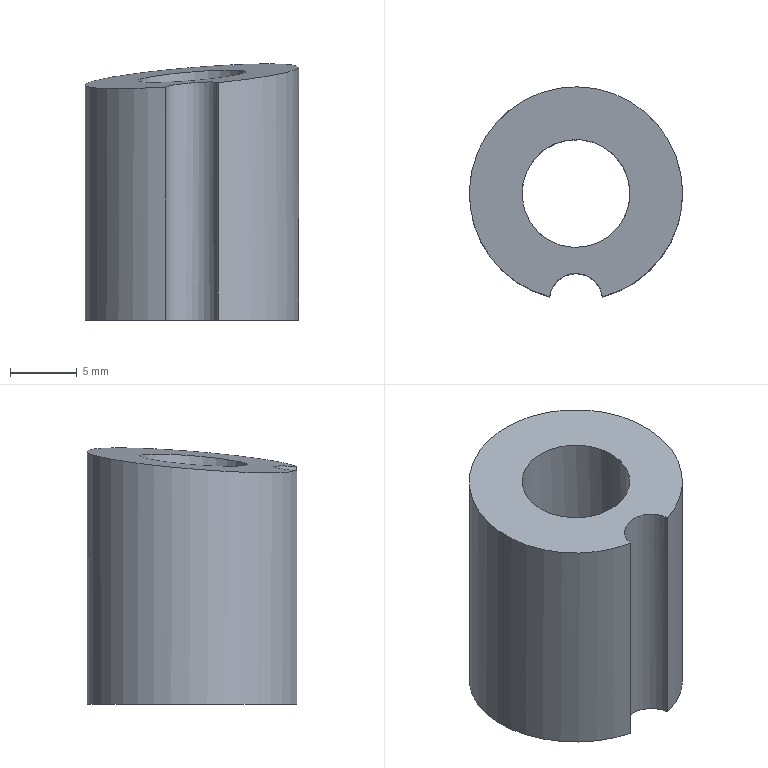Part | NX | features EKSD 16-20-8.100 2 | 1 solid | 7 faces | box 16 x 15.75 x 19.22 mm | volume 2189 mm3 | cylinder 4 | plane 3 | commonest cylinder face diameters 4 x1 8.1 x1 10.6 x1 16 x1
STEP:
#1=CARTESIAN_POINT('',(686.573,-10.452,-23.));
#2=VERTEX_POINT('',#1);
#3=CARTESIAN_POINT('',(682.604,-10.452,-23.));
#4=VERTEX_POINT('',#3);
#5=CARTESIAN_POINT('',(684.588,-10.702,-23.));
#6=DIRECTION('',(0.,0.,1.));
#7=DIRECTION('',(-1.,0.,0.));
#8=AXIS2_PLACEMENT_3D('',#5,#6,#7);
#9=CIRCLE('',#8,2.);
#10=EDGE_CURVE('',#2,#4,#9,.T.);
#11=ORIENTED_EDGE('',*,*,#10,.T.);
#12=CARTESIAN_POINT('',(684.588,-2.702,-23.));
#13=DIRECTION('',(0.,0.,1.));
#14=DIRECTION('',(-1.,0.,0.));
#15=AXIS2_PLACEMENT_3D('',#12,#13,#14);
#16=CIRCLE('',#15,8.);
#17=EDGE_CURVE('',#2,#4,#16,.T.);
#18=ORIENTED_EDGE('',*,*,#17,.F.);
#19=EDGE_LOOP('',(#11,#18));
#20=FACE_BOUND('',#19,.T.);
#21=CARTESIAN_POINT('',(689.888,-2.702,-23.));
#22=VERTEX_POINT('',#21);
#23=CARTESIAN_POINT('',(684.588,-2.702,-23.));
#24=DIRECTION('',(0.,0.,-1.));
#25=DIRECTION('',(1.,0.,0.));
#26=AXIS2_PLACEMENT_3D('',#23,#24,#25);
#27=CIRCLE('',#26,5.3);
#28=EDGE_CURVE('',#22,#22,#27,.T.);
#29=ORIENTED_EDGE('',*,*,#28,.F.);
#30=EDGE_LOOP('',(#29));
#31=FACE_BOUND('',#30,.T.);
#32=CARTESIAN_POINT('',(684.588,-2.702,-23.));
#33=DIRECTION('',(0.,0.,-1.));
#34=DIRECTION('',(1.,0.,0.));
#35=AXIS2_PLACEMENT_3D('',#32,#33,#34);
#36=PLANE('',#35);
#37=ADVANCED_FACE('',(#20,#31),#36,.T.);
#38=CARTESIAN_POINT('',(682.604,-10.452,-5.509));
#39=VERTEX_POINT('',#38);
#40=CARTESIAN_POINT('',(686.573,-10.452,-5.181));
#41=VERTEX_POINT('',#40);
#42=CARTESIAN_POINT('',(684.588,-10.702,-5.366));
#43=DIRECTION('',(0.08207,0.08131,-0.9933));
#44=DIRECTION('',(-0.7057,-0.6991,-0.1155));
#45=AXIS2_PLACEMENT_3D('',#42,#43,#44);
#46=ELLIPSE('',#45,2.013,2.);
#47=EDGE_CURVE('',#39,#41,#46,.T.);
#48=ORIENTED_EDGE('',*,*,#47,.T.);
#49=CARTESIAN_POINT('',(684.588,-2.702,-4.711));
#50=DIRECTION('',(0.08207,0.08131,-0.9933));
#51=DIRECTION('',(-0.7057,-0.6991,-0.1155));
#52=AXIS2_PLACEMENT_3D('',#49,#50,#51);
#53=ELLIPSE('',#52,8.054,8.);
#54=EDGE_CURVE('',#39,#41,#53,.T.);
#55=ORIENTED_EDGE('',*,*,#54,.F.);
#56=EDGE_LOOP('',(#48,#55));
#57=FACE_BOUND('',#56,.T.);
#58=CARTESIAN_POINT('',(681.711,-5.553,-5.182));
#59=VERTEX_POINT('',#58);
#60=CARTESIAN_POINT('',(684.588,-2.702,-4.711));
#61=DIRECTION('',(0.08207,0.08131,-0.9933));
#62=DIRECTION('',(-0.7057,-0.6991,-0.1155));
#63=AXIS2_PLACEMENT_3D('',#60,#61,#62);
#64=ELLIPSE('',#63,4.077,4.05);
#65=EDGE_CURVE('',#59,#59,#64,.F.);
#66=ORIENTED_EDGE('',*,*,#65,.F.);
#67=EDGE_LOOP('',(#66));
#68=FACE_BOUND('',#67,.T.);
#69=CARTESIAN_POINT('',(770.1,-94.991,-5.2));
#70=DIRECTION('',(0.08207,0.08131,-0.9933));
#71=DIRECTION('',(0.9966,-0.01117,0.08143));
#72=AXIS2_PLACEMENT_3D('',#69,#70,#71);
#73=PLANE('',#72);
#74=ADVANCED_FACE('',(#57,#68),#73,.F.);
#75=CARTESIAN_POINT('',(682.604,-10.452,-13.));
#76=DIRECTION('',(0.,0.,-1.));
#77=VECTOR('',#76,1000.);
#78=LINE('',#75,#77);
#79=EDGE_CURVE('',#39,#4,#78,.T.);
#80=ORIENTED_EDGE('',*,*,#79,.F.);
#81=ORIENTED_EDGE('',*,*,#54,.T.);
#82=CARTESIAN_POINT('',(686.573,-10.452,-13.));
#83=DIRECTION('',(0.,0.,-1.));
#84=VECTOR('',#83,1000.);
#85=LINE('',#82,#84);
#86=EDGE_CURVE('',#2,#41,#85,.F.);
#87=ORIENTED_EDGE('',*,*,#86,.F.);
#88=ORIENTED_EDGE('',*,*,#17,.T.);
#89=EDGE_LOOP('',(#80,#81,#87,#88));
#90=FACE_BOUND('',#89,.T.);
#91=CARTESIAN_POINT('',(684.588,-2.702,-3.));
#92=DIRECTION('',(0.,0.,-1.));
#93=DIRECTION('',(1.,0.,0.));
#94=AXIS2_PLACEMENT_3D('',#91,#92,#93);
#95=CYLINDRICAL_SURFACE('',#94,8.);
#96=ADVANCED_FACE('',(#90),#95,.T.);
#97=CARTESIAN_POINT('',(680.538,-2.702,-11.));
#98=VERTEX_POINT('',#97);
#99=CARTESIAN_POINT('',(684.588,-2.702,-11.));
#100=DIRECTION('',(0.,0.,1.));
#101=DIRECTION('',(-1.,0.,0.));
#102=AXIS2_PLACEMENT_3D('',#99,#100,#101);
#103=CIRCLE('',#102,4.05);
#104=EDGE_CURVE('',#98,#98,#103,.F.);
#105=ORIENTED_EDGE('',*,*,#104,.T.);
#106=EDGE_LOOP('',(#105));
#107=FACE_BOUND('',#106,.T.);
#108=ORIENTED_EDGE('',*,*,#65,.T.);
#109=EDGE_LOOP('',(#108));
#110=FACE_BOUND('',#109,.T.);
#111=CARTESIAN_POINT('',(684.588,-2.702,-2.));
#112=DIRECTION('',(0.,0.,-1.));
#113=DIRECTION('',(1.,0.,0.));
#114=AXIS2_PLACEMENT_3D('',#111,#112,#113);
#115=CYLINDRICAL_SURFACE('',#114,4.05);
#116=ADVANCED_FACE('',(#107,#110),#115,.F.);
#117=CARTESIAN_POINT('',(689.888,-2.702,-11.));
#118=VERTEX_POINT('',#117);
#119=CARTESIAN_POINT('',(684.588,-2.702,-11.));
#120=DIRECTION('',(0.,0.,-1.));
#121=DIRECTION('',(1.,0.,0.));
#122=AXIS2_PLACEMENT_3D('',#119,#120,#121);
#123=CIRCLE('',#122,5.3);
#124=EDGE_CURVE('',#118,#118,#123,.T.);
#125=ORIENTED_EDGE('',*,*,#124,.T.);
#126=EDGE_LOOP('',(#125));
#127=FACE_BOUND('',#126,.T.);
#128=ORIENTED_EDGE('',*,*,#104,.F.);
#129=EDGE_LOOP('',(#128));
#130=FACE_BOUND('',#129,.T.);
#131=CARTESIAN_POINT('',(684.588,-2.702,-11.));
#132=DIRECTION('',(0.,0.,1.));
#133=DIRECTION('',(-1.,0.,0.));
#134=AXIS2_PLACEMENT_3D('',#131,#132,#133);
#135=PLANE('',#134);
#136=ADVANCED_FACE('',(#127,#130),#135,.F.);
#137=ORIENTED_EDGE('',*,*,#28,.T.);
#138=EDGE_LOOP('',(#137));
#139=FACE_BOUND('',#138,.T.);
#140=ORIENTED_EDGE('',*,*,#124,.F.);
#141=EDGE_LOOP('',(#140));
#142=FACE_BOUND('',#141,.T.);
#143=CARTESIAN_POINT('',(684.588,-2.702,-11.));
#144=DIRECTION('',(0.,0.,-1.));
#145=DIRECTION('',(1.,0.,0.));
#146=AXIS2_PLACEMENT_3D('',#143,#144,#145);
#147=CYLINDRICAL_SURFACE('',#146,5.3);
#148=ADVANCED_FACE('',(#139,#142),#147,.F.);
#149=ORIENTED_EDGE('',*,*,#79,.T.);
#150=ORIENTED_EDGE('',*,*,#10,.F.);
#151=ORIENTED_EDGE('',*,*,#86,.T.);
#152=ORIENTED_EDGE('',*,*,#47,.F.);
#153=EDGE_LOOP('',(#149,#150,#151,#152));
#154=FACE_BOUND('',#153,.T.);
#155=CARTESIAN_POINT('',(684.588,-10.702,-3.));
#156=DIRECTION('',(0.,0.,-1.));
#157=DIRECTION('',(1.,0.,0.));
#158=AXIS2_PLACEMENT_3D('',#155,#156,#157);
#159=CYLINDRICAL_SURFACE('',#158,2.);
#160=ADVANCED_FACE('',(#154),#159,.F.);
#161=CLOSED_SHELL('',(#37,#74,#96,#116,#136,#148,#160));
#162=MANIFOLD_SOLID_BREP('',#161);
#163=(LENGTH_UNIT()NAMED_UNIT(*)SI_UNIT(.MILLI.,.METRE.));
#164=UNCERTAINTY_MEASURE_WITH_UNIT(LENGTH_MEASURE(0.00001),#163,'','');
#165=(NAMED_UNIT(*)PLANE_ANGLE_UNIT()SI_UNIT($,.RADIAN.));
#166=(NAMED_UNIT(*)SI_UNIT($,.STERADIAN.)SOLID_ANGLE_UNIT());
#167=(GEOMETRIC_REPRESENTATION_CONTEXT(3)GLOBAL_UNCERTAINTY_ASSIGNED_CONTEXT((#164))GLOBAL_UNIT_ASSIGNED_CONTEXT((#163,#165,#166))REPRESENTATION_CONTEXT('',''));
#168=ADVANCED_BREP_SHAPE_REPRESENTATION('',(#162),#167);